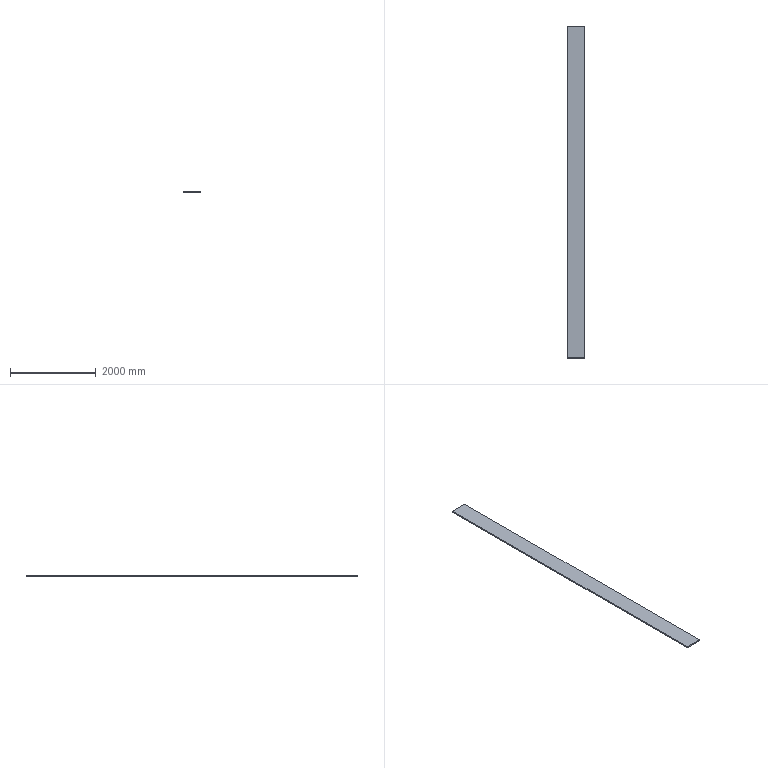Part | SolidWorks | features Extrusion 1 | 1 solid | 6 faces | box 400 x 7756 x 30 mm | volume 93072000 mm3 | plane 6
STEP:
#1=CARTESIAN_POINT('',(-200.,3878.,-15.));
#2=VERTEX_POINT('',#1);
#3=CARTESIAN_POINT('',(-200.,-3878.,-15.));
#4=VERTEX_POINT('',#3);
#5=CARTESIAN_POINT('',(-200.,3878.,-15.));
#6=DIRECTION('',(0.,-1.,0.));
#7=VECTOR('',#6,1000.);
#8=LINE('',#5,#7);
#9=EDGE_CURVE('',#2,#4,#8,.T.);
#10=ORIENTED_EDGE('',*,*,#9,.T.);
#11=CARTESIAN_POINT('',(-200.,-3878.,15.));
#12=VERTEX_POINT('',#11);
#13=CARTESIAN_POINT('',(-200.,-3878.,15.));
#14=DIRECTION('',(0.,0.,-1.));
#15=VECTOR('',#14,1000.);
#16=LINE('',#13,#15);
#17=EDGE_CURVE('',#12,#4,#16,.T.);
#18=ORIENTED_EDGE('',*,*,#17,.F.);
#19=CARTESIAN_POINT('',(-200.,3878.,15.));
#20=VERTEX_POINT('',#19);
#21=CARTESIAN_POINT('',(-200.,3878.,15.));
#22=DIRECTION('',(0.,-1.,0.));
#23=VECTOR('',#22,1000.);
#24=LINE('',#21,#23);
#25=EDGE_CURVE('',#20,#12,#24,.T.);
#26=ORIENTED_EDGE('',*,*,#25,.F.);
#27=CARTESIAN_POINT('',(-200.,3878.,15.));
#28=DIRECTION('',(0.,0.,-1.));
#29=VECTOR('',#28,1000.);
#30=LINE('',#27,#29);
#31=EDGE_CURVE('',#20,#2,#30,.T.);
#32=ORIENTED_EDGE('',*,*,#31,.T.);
#33=EDGE_LOOP('',(#10,#18,#26,#32));
#34=FACE_OUTER_BOUND('',#33,.T.);
#35=CARTESIAN_POINT('',(-200.,3878.,15.));
#36=DIRECTION('',(1.,0.,0.));
#37=DIRECTION('',(0.,1.,0.));
#38=AXIS2_PLACEMENT_3D('',#35,#36,#37);
#39=PLANE('',#38);
#40=ADVANCED_FACE('',(#34),#39,.F.);
#41=CARTESIAN_POINT('',(200.,-3878.,-15.));
#42=VERTEX_POINT('',#41);
#43=CARTESIAN_POINT('',(-200.,-3878.,-15.));
#44=DIRECTION('',(1.,0.,0.));
#45=VECTOR('',#44,1000.);
#46=LINE('',#43,#45);
#47=EDGE_CURVE('',#4,#42,#46,.T.);
#48=ORIENTED_EDGE('',*,*,#47,.T.);
#49=CARTESIAN_POINT('',(200.,-3878.,15.));
#50=VERTEX_POINT('',#49);
#51=CARTESIAN_POINT('',(200.,-3878.,15.));
#52=DIRECTION('',(0.,0.,-1.));
#53=VECTOR('',#52,1000.);
#54=LINE('',#51,#53);
#55=EDGE_CURVE('',#50,#42,#54,.T.);
#56=ORIENTED_EDGE('',*,*,#55,.F.);
#57=CARTESIAN_POINT('',(-200.,-3878.,15.));
#58=DIRECTION('',(1.,0.,0.));
#59=VECTOR('',#58,1000.);
#60=LINE('',#57,#59);
#61=EDGE_CURVE('',#12,#50,#60,.T.);
#62=ORIENTED_EDGE('',*,*,#61,.F.);
#63=ORIENTED_EDGE('',*,*,#17,.T.);
#64=EDGE_LOOP('',(#48,#56,#62,#63));
#65=FACE_OUTER_BOUND('',#64,.T.);
#66=CARTESIAN_POINT('',(-200.,-3878.,15.));
#67=DIRECTION('',(0.,1.,0.));
#68=DIRECTION('',(0.,0.,1.));
#69=AXIS2_PLACEMENT_3D('',#66,#67,#68);
#70=PLANE('',#69);
#71=ADVANCED_FACE('',(#65),#70,.F.);
#72=CARTESIAN_POINT('',(200.,3878.,-15.));
#73=VERTEX_POINT('',#72);
#74=CARTESIAN_POINT('',(200.,3878.,-15.));
#75=DIRECTION('',(0.,1.,0.));
#76=VECTOR('',#75,1000.);
#77=LINE('',#74,#76);
#78=EDGE_CURVE('',#42,#73,#77,.T.);
#79=ORIENTED_EDGE('',*,*,#78,.T.);
#80=CARTESIAN_POINT('',(200.,3878.,15.));
#81=VERTEX_POINT('',#80);
#82=CARTESIAN_POINT('',(200.,3878.,15.));
#83=DIRECTION('',(0.,0.,-1.));
#84=VECTOR('',#83,1000.);
#85=LINE('',#82,#84);
#86=EDGE_CURVE('',#81,#73,#85,.T.);
#87=ORIENTED_EDGE('',*,*,#86,.F.);
#88=CARTESIAN_POINT('',(200.,3878.,15.));
#89=DIRECTION('',(0.,1.,0.));
#90=VECTOR('',#89,1000.);
#91=LINE('',#88,#90);
#92=EDGE_CURVE('',#50,#81,#91,.T.);
#93=ORIENTED_EDGE('',*,*,#92,.F.);
#94=ORIENTED_EDGE('',*,*,#55,.T.);
#95=EDGE_LOOP('',(#79,#87,#93,#94));
#96=FACE_OUTER_BOUND('',#95,.T.);
#97=CARTESIAN_POINT('',(200.,3878.,15.));
#98=DIRECTION('',(-1.,0.,0.));
#99=DIRECTION('',(0.,-1.,0.));
#100=AXIS2_PLACEMENT_3D('',#97,#98,#99);
#101=PLANE('',#100);
#102=ADVANCED_FACE('',(#96),#101,.F.);
#103=CARTESIAN_POINT('',(-200.,3878.,-15.));
#104=DIRECTION('',(-1.,0.,0.));
#105=VECTOR('',#104,1000.);
#106=LINE('',#103,#105);
#107=EDGE_CURVE('',#73,#2,#106,.T.);
#108=ORIENTED_EDGE('',*,*,#107,.T.);
#109=ORIENTED_EDGE('',*,*,#31,.F.);
#110=CARTESIAN_POINT('',(-200.,3878.,15.));
#111=DIRECTION('',(-1.,0.,0.));
#112=VECTOR('',#111,1000.);
#113=LINE('',#110,#112);
#114=EDGE_CURVE('',#81,#20,#113,.T.);
#115=ORIENTED_EDGE('',*,*,#114,.F.);
#116=ORIENTED_EDGE('',*,*,#86,.T.);
#117=EDGE_LOOP('',(#108,#109,#115,#116));
#118=FACE_OUTER_BOUND('',#117,.T.);
#119=CARTESIAN_POINT('',(-200.,3878.,15.));
#120=DIRECTION('',(0.,-1.,0.));
#121=DIRECTION('',(0.,0.,-1.));
#122=AXIS2_PLACEMENT_3D('',#119,#120,#121);
#123=PLANE('',#122);
#124=ADVANCED_FACE('',(#118),#123,.F.);
#125=ORIENTED_EDGE('',*,*,#25,.T.);
#126=ORIENTED_EDGE('',*,*,#61,.T.);
#127=ORIENTED_EDGE('',*,*,#92,.T.);
#128=ORIENTED_EDGE('',*,*,#114,.T.);
#129=EDGE_LOOP('',(#125,#126,#127,#128));
#130=FACE_OUTER_BOUND('',#129,.T.);
#131=CARTESIAN_POINT('',(-200.,-3878.,15.));
#132=DIRECTION('',(0.,0.,1.));
#133=DIRECTION('',(1.,0.,0.));
#134=AXIS2_PLACEMENT_3D('',#131,#132,#133);
#135=PLANE('',#134);
#136=ADVANCED_FACE('',(#130),#135,.T.);
#137=ORIENTED_EDGE('',*,*,#9,.F.);
#138=ORIENTED_EDGE('',*,*,#107,.F.);
#139=ORIENTED_EDGE('',*,*,#78,.F.);
#140=ORIENTED_EDGE('',*,*,#47,.F.);
#141=EDGE_LOOP('',(#137,#138,#139,#140));
#142=FACE_OUTER_BOUND('',#141,.T.);
#143=CARTESIAN_POINT('',(-200.,-3878.,-15.));
#144=DIRECTION('',(0.,0.,1.));
#145=DIRECTION('',(1.,0.,0.));
#146=AXIS2_PLACEMENT_3D('',#143,#144,#145);
#147=PLANE('',#146);
#148=ADVANCED_FACE('',(#142),#147,.F.);
#149=CLOSED_SHELL('',(#40,#71,#102,#124,#136,#148));
#150=MANIFOLD_SOLID_BREP('',#149);
#151=CARTESIAN_POINT('',(0.,0.,0.));
#152=DIRECTION('',(0.,0.,1.));
#153=DIRECTION('',(1.,0.,0.));
#154=AXIS2_PLACEMENT_3D('',#151,#152,#153);
#155=(LENGTH_UNIT()NAMED_UNIT(*)SI_UNIT(.MILLI.,.METRE.));
#156=UNCERTAINTY_MEASURE_WITH_UNIT(LENGTH_MEASURE(0.00001),#155,'','');
#157=(NAMED_UNIT(*)PLANE_ANGLE_UNIT()SI_UNIT($,.RADIAN.));
#158=(NAMED_UNIT(*)SI_UNIT($,.STERADIAN.)SOLID_ANGLE_UNIT());
#159=(GEOMETRIC_REPRESENTATION_CONTEXT(3)GLOBAL_UNCERTAINTY_ASSIGNED_CONTEXT((#156))GLOBAL_UNIT_ASSIGNED_CONTEXT((#155,#157,#158))REPRESENTATION_CONTEXT('',''));
#160=ADVANCED_BREP_SHAPE_REPRESENTATION('',(#150,#154),#159);